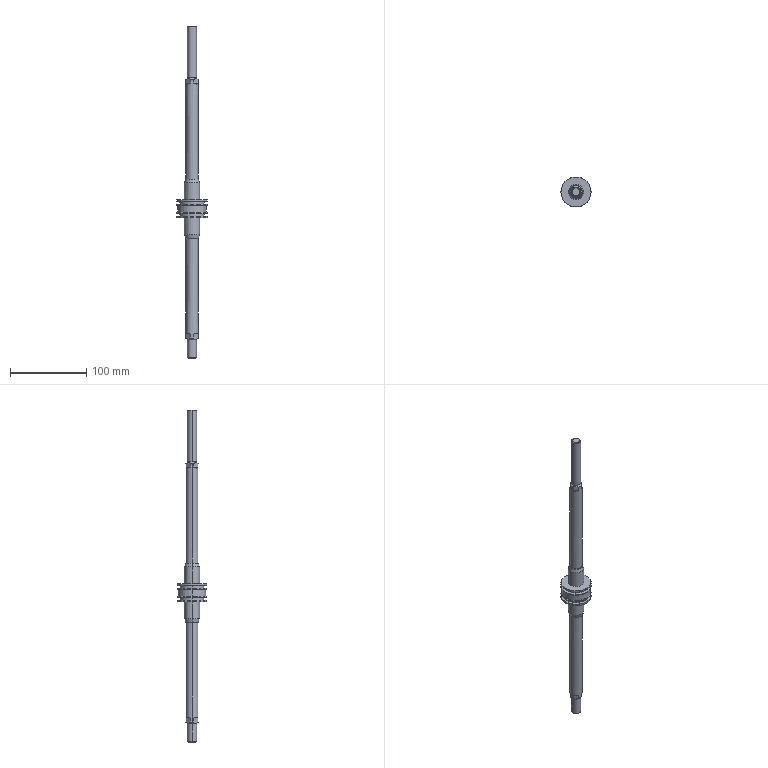Part | SolidWorks | features BaseBody 1 | 1 solid | 90 faces | box 39.5 x 39.5 x 435 mm | volume 104659 mm3 | cone 28 | plane 28 | cylinder 26 | torus 8 | commonest cylinder face diameters 39.5 x8 12 x4 16 x4 20 x4 32 x4 36.9 x2